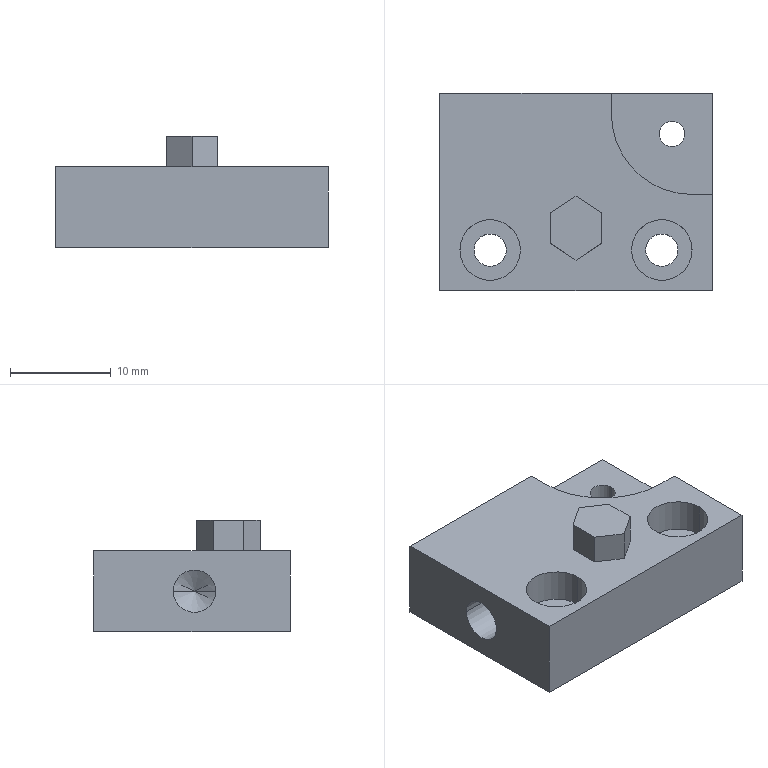Part | NX | 1 solid | 33 faces | box 27 x 19.5 x 11 mm | volume 3556 mm3 | plane 18 | cylinder 13 | cone 2 | commonest cylinder face diameters 3.2 x4 6 x4 2.5 x2 4.2 x2 16 x1
STEP:
#1=CARTESIAN_POINT('',(27.,0.,0.));
#2=VERTEX_POINT('',#1);
#3=CARTESIAN_POINT('',(0.,0.,0.));
#4=VERTEX_POINT('',#3);
#5=CARTESIAN_POINT('',(27.,0.,0.));
#6=DIRECTION('',(-1.,0.,0.));
#7=VECTOR('',#6,1000.);
#8=LINE('',#5,#7);
#9=EDGE_CURVE('',#2,#4,#8,.T.);
#10=ORIENTED_EDGE('',*,*,#9,.T.);
#11=CARTESIAN_POINT('',(0.,19.5,0.));
#12=VERTEX_POINT('',#11);
#13=CARTESIAN_POINT('',(0.,0.,0.));
#14=DIRECTION('',(0.,1.,0.));
#15=VECTOR('',#14,1000.);
#16=LINE('',#13,#15);
#17=EDGE_CURVE('',#4,#12,#16,.T.);
#18=ORIENTED_EDGE('',*,*,#17,.T.);
#19=CARTESIAN_POINT('',(27.,19.5,0.));
#20=VERTEX_POINT('',#19);
#21=CARTESIAN_POINT('',(0.,19.5,0.));
#22=DIRECTION('',(1.,0.,0.));
#23=VECTOR('',#22,1000.);
#24=LINE('',#21,#23);
#25=EDGE_CURVE('',#12,#20,#24,.T.);
#26=ORIENTED_EDGE('',*,*,#25,.T.);
#27=CARTESIAN_POINT('',(27.,19.5,0.));
#28=DIRECTION('',(0.,-1.,0.));
#29=VECTOR('',#28,1000.);
#30=LINE('',#27,#29);
#31=EDGE_CURVE('',#20,#2,#30,.T.);
#32=ORIENTED_EDGE('',*,*,#31,.T.);
#33=EDGE_LOOP('',(#10,#18,#26,#32));
#34=FACE_BOUND('',#33,.T.);
#35=CARTESIAN_POINT('',(6.6,4.,0.));
#36=VERTEX_POINT('',#35);
#37=CARTESIAN_POINT('',(3.4,4.,0.));
#38=VERTEX_POINT('',#37);
#39=CARTESIAN_POINT('',(5.,4.,0.));
#40=DIRECTION('',(0.,0.,-1.));
#41=DIRECTION('',(-1.,0.,0.));
#42=AXIS2_PLACEMENT_3D('',#39,#40,#41);
#43=CIRCLE('',#42,1.6);
#44=EDGE_CURVE('',#36,#38,#43,.T.);
#45=ORIENTED_EDGE('',*,*,#44,.F.);
#46=CARTESIAN_POINT('',(5.,4.,0.));
#47=DIRECTION('',(0.,0.,-1.));
#48=DIRECTION('',(-1.,0.,0.));
#49=AXIS2_PLACEMENT_3D('',#46,#47,#48);
#50=CIRCLE('',#49,1.6);
#51=EDGE_CURVE('',#38,#36,#50,.T.);
#52=ORIENTED_EDGE('',*,*,#51,.F.);
#53=EDGE_LOOP('',(#45,#52));
#54=FACE_BOUND('',#53,.T.);
#55=CARTESIAN_POINT('',(23.6,4.,0.));
#56=VERTEX_POINT('',#55);
#57=CARTESIAN_POINT('',(20.4,4.,0.));
#58=VERTEX_POINT('',#57);
#59=CARTESIAN_POINT('',(22.,4.,0.));
#60=DIRECTION('',(0.,0.,-1.));
#61=DIRECTION('',(-1.,0.,0.));
#62=AXIS2_PLACEMENT_3D('',#59,#60,#61);
#63=CIRCLE('',#62,1.6);
#64=EDGE_CURVE('',#56,#58,#63,.T.);
#65=ORIENTED_EDGE('',*,*,#64,.F.);
#66=CARTESIAN_POINT('',(22.,4.,0.));
#67=DIRECTION('',(0.,0.,-1.));
#68=DIRECTION('',(-1.,0.,0.));
#69=AXIS2_PLACEMENT_3D('',#66,#67,#68);
#70=CIRCLE('',#69,1.6);
#71=EDGE_CURVE('',#58,#56,#70,.T.);
#72=ORIENTED_EDGE('',*,*,#71,.F.);
#73=EDGE_LOOP('',(#65,#72));
#74=FACE_BOUND('',#73,.T.);
#75=CARTESIAN_POINT('',(24.25,15.5,0.));
#76=VERTEX_POINT('',#75);
#77=CARTESIAN_POINT('',(21.75,15.5,0.));
#78=VERTEX_POINT('',#77);
#79=CARTESIAN_POINT('',(23.,15.5,0.));
#80=DIRECTION('',(0.,0.,-1.));
#81=DIRECTION('',(-1.,0.,0.));
#82=AXIS2_PLACEMENT_3D('',#79,#80,#81);
#83=CIRCLE('',#82,1.25);
#84=EDGE_CURVE('',#76,#78,#83,.T.);
#85=ORIENTED_EDGE('',*,*,#84,.F.);
#86=CARTESIAN_POINT('',(23.,15.5,0.));
#87=DIRECTION('',(0.,0.,-1.));
#88=DIRECTION('',(-1.,0.,0.));
#89=AXIS2_PLACEMENT_3D('',#86,#87,#88);
#90=CIRCLE('',#89,1.25);
#91=EDGE_CURVE('',#78,#76,#90,.T.);
#92=ORIENTED_EDGE('',*,*,#91,.F.);
#93=EDGE_LOOP('',(#85,#92));
#94=FACE_BOUND('',#93,.T.);
#95=CARTESIAN_POINT('',(0.,0.,0.));
#96=DIRECTION('',(0.,0.,1.));
#97=DIRECTION('',(1.,0.,0.));
#98=AXIS2_PLACEMENT_3D('',#95,#96,#97);
#99=PLANE('',#98);
#100=ADVANCED_FACE('',(#34,#54,#74,#94),#99,.F.);
#101=ORIENTED_EDGE('',*,*,#9,.F.);
#102=CARTESIAN_POINT('',(27.,0.,8.));
#103=VERTEX_POINT('',#102);
#104=CARTESIAN_POINT('',(27.,0.,8.));
#105=DIRECTION('',(0.,0.,-1.));
#106=VECTOR('',#105,1000.);
#107=LINE('',#104,#106);
#108=EDGE_CURVE('',#103,#2,#107,.T.);
#109=ORIENTED_EDGE('',*,*,#108,.F.);
#110=CARTESIAN_POINT('',(0.,0.,8.));
#111=VERTEX_POINT('',#110);
#112=CARTESIAN_POINT('',(27.,0.,8.));
#113=DIRECTION('',(-1.,0.,0.));
#114=VECTOR('',#113,1000.);
#115=LINE('',#112,#114);
#116=EDGE_CURVE('',#103,#111,#115,.T.);
#117=ORIENTED_EDGE('',*,*,#116,.T.);
#118=CARTESIAN_POINT('',(0.,0.,8.));
#119=DIRECTION('',(0.,0.,-1.));
#120=VECTOR('',#119,1000.);
#121=LINE('',#118,#120);
#122=EDGE_CURVE('',#111,#4,#121,.T.);
#123=ORIENTED_EDGE('',*,*,#122,.T.);
#124=EDGE_LOOP('',(#101,#109,#117,#123));
#125=FACE_BOUND('',#124,.T.);
#126=CARTESIAN_POINT('',(0.,0.,0.));
#127=DIRECTION('',(0.,-1.,0.));
#128=DIRECTION('',(0.,0.,-1.));
#129=AXIS2_PLACEMENT_3D('',#126,#127,#128);
#130=PLANE('',#129);
#131=ADVANCED_FACE('',(#125),#130,.T.);
#132=ORIENTED_EDGE('',*,*,#17,.F.);
#133=ORIENTED_EDGE('',*,*,#122,.F.);
#134=CARTESIAN_POINT('',(0.,19.5,8.));
#135=VERTEX_POINT('',#134);
#136=CARTESIAN_POINT('',(0.,0.,8.));
#137=DIRECTION('',(0.,1.,0.));
#138=VECTOR('',#137,1000.);
#139=LINE('',#136,#138);
#140=EDGE_CURVE('',#111,#135,#139,.T.);
#141=ORIENTED_EDGE('',*,*,#140,.T.);
#142=CARTESIAN_POINT('',(0.,19.5,8.));
#143=DIRECTION('',(0.,0.,-1.));
#144=VECTOR('',#143,1000.);
#145=LINE('',#142,#144);
#146=EDGE_CURVE('',#135,#12,#145,.T.);
#147=ORIENTED_EDGE('',*,*,#146,.T.);
#148=EDGE_LOOP('',(#132,#133,#141,#147));
#149=FACE_BOUND('',#148,.T.);
#150=CARTESIAN_POINT('',(0.,11.6,4.));
#151=VERTEX_POINT('',#150);
#152=CARTESIAN_POINT('',(0.,7.4,4.));
#153=VERTEX_POINT('',#152);
#154=CARTESIAN_POINT('',(0.,9.5,4.));
#155=DIRECTION('',(-1.,0.,0.));
#156=DIRECTION('',(0.,-1.,0.));
#157=AXIS2_PLACEMENT_3D('',#154,#155,#156);
#158=CIRCLE('',#157,2.1);
#159=EDGE_CURVE('',#151,#153,#158,.T.);
#160=ORIENTED_EDGE('',*,*,#159,.F.);
#161=CARTESIAN_POINT('',(0.,9.5,4.));
#162=DIRECTION('',(-1.,0.,0.));
#163=DIRECTION('',(0.,-1.,0.));
#164=AXIS2_PLACEMENT_3D('',#161,#162,#163);
#165=CIRCLE('',#164,2.1);
#166=EDGE_CURVE('',#153,#151,#165,.T.);
#167=ORIENTED_EDGE('',*,*,#166,.F.);
#168=EDGE_LOOP('',(#160,#167));
#169=FACE_BOUND('',#168,.T.);
#170=CARTESIAN_POINT('',(0.,19.5,0.));
#171=DIRECTION('',(-1.,0.,0.));
#172=DIRECTION('',(0.,0.,1.));
#173=AXIS2_PLACEMENT_3D('',#170,#171,#172);
#174=PLANE('',#173);
#175=ADVANCED_FACE('',(#149,#169),#174,.T.);
#176=CARTESIAN_POINT('',(17.,19.5,5.));
#177=VERTEX_POINT('',#176);
#178=CARTESIAN_POINT('',(27.,19.5,5.));
#179=VERTEX_POINT('',#178);
#180=CARTESIAN_POINT('',(17.,19.5,5.));
#181=DIRECTION('',(1.,0.,0.));
#182=VECTOR('',#181,1000.);
#183=LINE('',#180,#182);
#184=EDGE_CURVE('',#177,#179,#183,.T.);
#185=ORIENTED_EDGE('',*,*,#184,.T.);
#186=CARTESIAN_POINT('',(27.,19.5,5.));
#187=DIRECTION('',(0.,0.,-1.));
#188=VECTOR('',#187,1000.);
#189=LINE('',#186,#188);
#190=EDGE_CURVE('',#179,#20,#189,.T.);
#191=ORIENTED_EDGE('',*,*,#190,.T.);
#192=ORIENTED_EDGE('',*,*,#25,.F.);
#193=ORIENTED_EDGE('',*,*,#146,.F.);
#194=CARTESIAN_POINT('',(17.,19.5,8.));
#195=VERTEX_POINT('',#194);
#196=CARTESIAN_POINT('',(0.,19.5,8.));
#197=DIRECTION('',(1.,0.,0.));
#198=VECTOR('',#197,1000.);
#199=LINE('',#196,#198);
#200=EDGE_CURVE('',#135,#195,#199,.T.);
#201=ORIENTED_EDGE('',*,*,#200,.T.);
#202=CARTESIAN_POINT('',(17.,19.5,5.));
#203=DIRECTION('',(0.,0.,1.));
#204=VECTOR('',#203,1000.);
#205=LINE('',#202,#204);
#206=EDGE_CURVE('',#177,#195,#205,.T.);
#207=ORIENTED_EDGE('',*,*,#206,.F.);
#208=EDGE_LOOP('',(#185,#191,#192,#193,#201,#207));
#209=FACE_BOUND('',#208,.T.);
#210=CARTESIAN_POINT('',(27.,19.5,0.));
#211=DIRECTION('',(0.,1.,0.));
#212=DIRECTION('',(1.,0.,0.));
#213=AXIS2_PLACEMENT_3D('',#210,#211,#212);
#214=PLANE('',#213);
#215=ADVANCED_FACE('',(#209),#214,.T.);
#216=CARTESIAN_POINT('',(27.,9.5,5.));
#217=VERTEX_POINT('',#216);
#218=CARTESIAN_POINT('',(27.,9.5,5.));
#219=DIRECTION('',(0.,1.,0.));
#220=VECTOR('',#219,1000.);
#221=LINE('',#218,#220);
#222=EDGE_CURVE('',#217,#179,#221,.T.);
#223=ORIENTED_EDGE('',*,*,#222,.T.);
#224=ORIENTED_EDGE('',*,*,#184,.F.);
#225=CARTESIAN_POINT('',(17.,17.5,5.));
#226=VERTEX_POINT('',#225);
#227=CARTESIAN_POINT('',(17.,17.5,5.));
#228=DIRECTION('',(0.,1.,0.));
#229=VECTOR('',#228,1000.);
#230=LINE('',#227,#229);
#231=EDGE_CURVE('',#226,#177,#230,.T.);
#232=ORIENTED_EDGE('',*,*,#231,.F.);
#233=CARTESIAN_POINT('',(25.,9.5,5.));
#234=VERTEX_POINT('',#233);
#235=CARTESIAN_POINT('',(25.,17.5,5.));
#236=DIRECTION('',(0.,0.,-1.));
#237=DIRECTION('',(0.,-1.,0.));
#238=AXIS2_PLACEMENT_3D('',#235,#236,#237);
#239=CIRCLE('',#238,8.);
#240=EDGE_CURVE('',#234,#226,#239,.T.);
#241=ORIENTED_EDGE('',*,*,#240,.F.);
#242=CARTESIAN_POINT('',(27.,9.5,5.));
#243=DIRECTION('',(-1.,0.,0.));
#244=VECTOR('',#243,1000.);
#245=LINE('',#242,#244);
#246=EDGE_CURVE('',#217,#234,#245,.T.);
#247=ORIENTED_EDGE('',*,*,#246,.F.);
#248=EDGE_LOOP('',(#223,#224,#232,#241,#247));
#249=FACE_BOUND('',#248,.T.);
#250=CARTESIAN_POINT('',(24.25,15.5,5.));
#251=VERTEX_POINT('',#250);
#252=CARTESIAN_POINT('',(21.75,15.5,5.));
#253=VERTEX_POINT('',#252);
#254=CARTESIAN_POINT('',(23.,15.5,5.));
#255=DIRECTION('',(0.,0.,1.));
#256=DIRECTION('',(1.,0.,0.));
#257=AXIS2_PLACEMENT_3D('',#254,#255,#256);
#258=CIRCLE('',#257,1.25);
#259=EDGE_CURVE('',#251,#253,#258,.T.);
#260=ORIENTED_EDGE('',*,*,#259,.F.);
#261=CARTESIAN_POINT('',(23.,15.5,5.));
#262=DIRECTION('',(0.,0.,1.));
#263=DIRECTION('',(1.,0.,0.));
#264=AXIS2_PLACEMENT_3D('',#261,#262,#263);
#265=CIRCLE('',#264,1.25);
#266=EDGE_CURVE('',#253,#251,#265,.T.);
#267=ORIENTED_EDGE('',*,*,#266,.F.);
#268=EDGE_LOOP('',(#260,#267));
#269=FACE_BOUND('',#268,.T.);
#270=CARTESIAN_POINT('',(0.,0.,5.));
#271=DIRECTION('',(0.,0.,1.));
#272=DIRECTION('',(1.,0.,0.));
#273=AXIS2_PLACEMENT_3D('',#270,#271,#272);
#274=PLANE('',#273);
#275=ADVANCED_FACE('',(#249,#269),#274,.T.);
#276=ORIENTED_EDGE('',*,*,#222,.F.);
#277=CARTESIAN_POINT('',(27.,9.5,8.));
#278=VERTEX_POINT('',#277);
#279=CARTESIAN_POINT('',(27.,9.5,5.));
#280=DIRECTION('',(0.,0.,1.));
#281=VECTOR('',#280,1000.);
#282=LINE('',#279,#281);
#283=EDGE_CURVE('',#217,#278,#282,.T.);
#284=ORIENTED_EDGE('',*,*,#283,.T.);
#285=CARTESIAN_POINT('',(27.,9.5,8.));
#286=DIRECTION('',(0.,-1.,0.));
#287=VECTOR('',#286,1000.);
#288=LINE('',#285,#287);
#289=EDGE_CURVE('',#278,#103,#288,.T.);
#290=ORIENTED_EDGE('',*,*,#289,.T.);
#291=ORIENTED_EDGE('',*,*,#108,.T.);
#292=ORIENTED_EDGE('',*,*,#31,.F.);
#293=ORIENTED_EDGE('',*,*,#190,.F.);
#294=EDGE_LOOP('',(#276,#284,#290,#291,#292,#293));
#295=FACE_BOUND('',#294,.T.);
#296=CARTESIAN_POINT('',(27.,0.,0.));
#297=DIRECTION('',(1.,0.,0.));
#298=DIRECTION('',(0.,1.,0.));
#299=AXIS2_PLACEMENT_3D('',#296,#297,#298);
#300=PLANE('',#299);
#301=ADVANCED_FACE('',(#295),#300,.T.);
#302=CARTESIAN_POINT('',(17.,17.5,8.));
#303=VERTEX_POINT('',#302);
#304=CARTESIAN_POINT('',(17.,17.5,8.));
#305=DIRECTION('',(0.,1.,0.));
#306=VECTOR('',#305,1000.);
#307=LINE('',#304,#306);
#308=EDGE_CURVE('',#303,#195,#307,.T.);
#309=ORIENTED_EDGE('',*,*,#308,.T.);
#310=ORIENTED_EDGE('',*,*,#200,.F.);
#311=ORIENTED_EDGE('',*,*,#140,.F.);
#312=ORIENTED_EDGE('',*,*,#116,.F.);
#313=ORIENTED_EDGE('',*,*,#289,.F.);
#314=CARTESIAN_POINT('',(25.,9.5,8.));
#315=VERTEX_POINT('',#314);
#316=CARTESIAN_POINT('',(25.,9.5,8.));
#317=DIRECTION('',(1.,0.,0.));
#318=VECTOR('',#317,1000.);
#319=LINE('',#316,#318);
#320=EDGE_CURVE('',#315,#278,#319,.T.);
#321=ORIENTED_EDGE('',*,*,#320,.F.);
#322=CARTESIAN_POINT('',(25.,17.5,8.));
#323=DIRECTION('',(0.,0.,1.));
#324=DIRECTION('',(-1.,0.,0.));
#325=AXIS2_PLACEMENT_3D('',#322,#323,#324);
#326=CIRCLE('',#325,8.);
#327=EDGE_CURVE('',#303,#315,#326,.T.);
#328=ORIENTED_EDGE('',*,*,#327,.F.);
#329=EDGE_LOOP('',(#309,#310,#311,#312,#313,#321,#328));
#330=FACE_BOUND('',#329,.T.);
#331=CARTESIAN_POINT('',(8.,4.,8.));
#332=VERTEX_POINT('',#331);
#333=CARTESIAN_POINT('',(2.,4.,8.));
#334=VERTEX_POINT('',#333);
#335=CARTESIAN_POINT('',(5.,4.,8.));
#336=DIRECTION('',(0.,0.,1.));
#337=DIRECTION('',(1.,0.,0.));
#338=AXIS2_PLACEMENT_3D('',#335,#336,#337);
#339=CIRCLE('',#338,3.);
#340=EDGE_CURVE('',#332,#334,#339,.T.);
#341=ORIENTED_EDGE('',*,*,#340,.F.);
#342=CARTESIAN_POINT('',(5.,4.,8.));
#343=DIRECTION('',(0.,0.,1.));
#344=DIRECTION('',(1.,0.,0.));
#345=AXIS2_PLACEMENT_3D('',#342,#343,#344);
#346=CIRCLE('',#345,3.);
#347=EDGE_CURVE('',#334,#332,#346,.T.);
#348=ORIENTED_EDGE('',*,*,#347,.F.);
#349=EDGE_LOOP('',(#341,#348));
#350=FACE_BOUND('',#349,.T.);
#351=CARTESIAN_POINT('',(19.,4.,8.));
#352=VERTEX_POINT('',#351);
#353=CARTESIAN_POINT('',(25.,4.,8.));
#354=VERTEX_POINT('',#353);
#355=CARTESIAN_POINT('',(22.,4.,8.));
#356=DIRECTION('',(0.,0.,1.));
#357=DIRECTION('',(1.,0.,0.));
#358=AXIS2_PLACEMENT_3D('',#355,#356,#357);
#359=CIRCLE('',#358,3.);
#360=EDGE_CURVE('',#352,#354,#359,.T.);
#361=ORIENTED_EDGE('',*,*,#360,.F.);
#362=CARTESIAN_POINT('',(22.,4.,8.));
#363=DIRECTION('',(0.,0.,1.));
#364=DIRECTION('',(1.,0.,0.));
#365=AXIS2_PLACEMENT_3D('',#362,#363,#364);
#366=CIRCLE('',#365,3.);
#367=EDGE_CURVE('',#354,#352,#366,.T.);
#368=ORIENTED_EDGE('',*,*,#367,.F.);
#369=EDGE_LOOP('',(#361,#368));
#370=FACE_BOUND('',#369,.T.);
#371=CARTESIAN_POINT('',(13.5,9.317,8.));
#372=VERTEX_POINT('',#371);
#373=CARTESIAN_POINT('',(11.,7.658,8.));
#374=VERTEX_POINT('',#373);
#375=CARTESIAN_POINT('',(13.5,9.317,8.));
#376=DIRECTION('',(-0.8333,-0.5528,0.));
#377=VECTOR('',#376,1000.);
#378=LINE('',#375,#377);
#379=EDGE_CURVE('',#372,#374,#378,.T.);
#380=ORIENTED_EDGE('',*,*,#379,.F.);
#381=CARTESIAN_POINT('',(16.,7.658,8.));
#382=VERTEX_POINT('',#381);
#383=CARTESIAN_POINT('',(16.,7.658,8.));
#384=DIRECTION('',(-0.8333,0.5528,0.));
#385=VECTOR('',#384,1000.);
#386=LINE('',#383,#385);
#387=EDGE_CURVE('',#382,#372,#386,.T.);
#388=ORIENTED_EDGE('',*,*,#387,.F.);
#389=CARTESIAN_POINT('',(16.,4.658,8.));
#390=VERTEX_POINT('',#389);
#391=CARTESIAN_POINT('',(16.,7.658,8.));
#392=DIRECTION('',(0.,-1.,0.));
#393=VECTOR('',#392,1000.);
#394=LINE('',#391,#393);
#395=EDGE_CURVE('',#382,#390,#394,.T.);
#396=ORIENTED_EDGE('',*,*,#395,.T.);
#397=CARTESIAN_POINT('',(13.5,3.,8.));
#398=VERTEX_POINT('',#397);
#399=CARTESIAN_POINT('',(13.5,3.,8.));
#400=DIRECTION('',(0.8333,0.5528,0.));
#401=VECTOR('',#400,1000.);
#402=LINE('',#399,#401);
#403=EDGE_CURVE('',#398,#390,#402,.T.);
#404=ORIENTED_EDGE('',*,*,#403,.F.);
#405=CARTESIAN_POINT('',(11.,4.658,8.));
#406=VERTEX_POINT('',#405);
#407=CARTESIAN_POINT('',(11.,4.658,8.));
#408=DIRECTION('',(0.8333,-0.5528,0.));
#409=VECTOR('',#408,1000.);
#410=LINE('',#407,#409);
#411=EDGE_CURVE('',#406,#398,#410,.T.);
#412=ORIENTED_EDGE('',*,*,#411,.F.);
#413=CARTESIAN_POINT('',(11.,4.658,8.));
#414=DIRECTION('',(0.,1.,0.));
#415=VECTOR('',#414,1000.);
#416=LINE('',#413,#415);
#417=EDGE_CURVE('',#406,#374,#416,.T.);
#418=ORIENTED_EDGE('',*,*,#417,.T.);
#419=EDGE_LOOP('',(#380,#388,#396,#404,#412,#418));
#420=FACE_BOUND('',#419,.T.);
#421=CARTESIAN_POINT('',(0.,0.,8.));
#422=DIRECTION('',(0.,0.,1.));
#423=DIRECTION('',(1.,0.,0.));
#424=AXIS2_PLACEMENT_3D('',#421,#422,#423);
#425=PLANE('',#424);
#426=ADVANCED_FACE('',(#330,#350,#370,#420),#425,.T.);
#427=ORIENTED_EDGE('',*,*,#308,.F.);
#428=CARTESIAN_POINT('',(17.,17.5,8.));
#429=DIRECTION('',(0.,0.,1.));
#430=VECTOR('',#429,1000.);
#431=LINE('',#428,#430);
#432=EDGE_CURVE('',#226,#303,#431,.T.);
#433=ORIENTED_EDGE('',*,*,#432,.F.);
#434=ORIENTED_EDGE('',*,*,#231,.T.);
#435=ORIENTED_EDGE('',*,*,#206,.T.);
#436=EDGE_LOOP('',(#427,#433,#434,#435));
#437=FACE_BOUND('',#436,.T.);
#438=CARTESIAN_POINT('',(17.,19.5,8.));
#439=DIRECTION('',(-1.,0.,0.));
#440=DIRECTION('',(0.,0.,1.));
#441=AXIS2_PLACEMENT_3D('',#438,#439,#440);
#442=PLANE('',#441);
#443=ADVANCED_FACE('',(#437),#442,.F.);
#444=ORIENTED_EDGE('',*,*,#327,.T.);
#445=CARTESIAN_POINT('',(25.,9.5,5.));
#446=DIRECTION('',(0.,0.,1.));
#447=VECTOR('',#446,1000.);
#448=LINE('',#445,#447);
#449=EDGE_CURVE('',#234,#315,#448,.T.);
#450=ORIENTED_EDGE('',*,*,#449,.F.);
#451=ORIENTED_EDGE('',*,*,#240,.T.);
#452=ORIENTED_EDGE('',*,*,#432,.T.);
#453=EDGE_LOOP('',(#444,#450,#451,#452));
#454=FACE_BOUND('',#453,.T.);
#455=CARTESIAN_POINT('',(25.,17.5,8.));
#456=DIRECTION('',(0.,0.,1.));
#457=DIRECTION('',(1.,0.,0.));
#458=AXIS2_PLACEMENT_3D('',#455,#456,#457);
#459=CYLINDRICAL_SURFACE('',#458,8.);
#460=ADVANCED_FACE('',(#454),#459,.F.);
#461=ORIENTED_EDGE('',*,*,#320,.T.);
#462=ORIENTED_EDGE('',*,*,#283,.F.);
#463=ORIENTED_EDGE('',*,*,#246,.T.);
#464=ORIENTED_EDGE('',*,*,#449,.T.);
#465=EDGE_LOOP('',(#461,#462,#463,#464));
#466=FACE_BOUND('',#465,.T.);
#467=CARTESIAN_POINT('',(25.,9.5,8.));
#468=DIRECTION('',(0.,-1.,0.));
#469=DIRECTION('',(0.,0.,-1.));
#470=AXIS2_PLACEMENT_3D('',#467,#468,#469);
#471=PLANE('',#470);
#472=ADVANCED_FACE('',(#466),#471,.F.);
#473=CARTESIAN_POINT('',(2.,4.,4.7));
#474=VERTEX_POINT('',#473);
#475=CARTESIAN_POINT('',(8.,4.,4.7));
#476=VERTEX_POINT('',#475);
#477=CARTESIAN_POINT('',(5.,4.,4.7));
#478=DIRECTION('',(0.,0.,-1.));
#479=DIRECTION('',(-1.,0.,0.));
#480=AXIS2_PLACEMENT_3D('',#477,#478,#479);
#481=CIRCLE('',#480,3.);
#482=EDGE_CURVE('',#474,#476,#481,.T.);
#483=ORIENTED_EDGE('',*,*,#482,.T.);
#484=CARTESIAN_POINT('',(8.,4.,-1.24));
#485=DIRECTION('',(0.,0.,1.));
#486=VECTOR('',#485,1000.);
#487=LINE('',#484,#486);
#488=EDGE_CURVE('',#332,#476,#487,.F.);
#489=ORIENTED_EDGE('',*,*,#488,.F.);
#490=ORIENTED_EDGE('',*,*,#340,.T.);
#491=CARTESIAN_POINT('',(2.,4.,-1.24));
#492=DIRECTION('',(0.,0.,1.));
#493=VECTOR('',#492,1000.);
#494=LINE('',#491,#493);
#495=EDGE_CURVE('',#334,#474,#494,.F.);
#496=ORIENTED_EDGE('',*,*,#495,.T.);
#497=EDGE_LOOP('',(#483,#489,#490,#496));
#498=FACE_BOUND('',#497,.T.);
#499=CARTESIAN_POINT('',(5.,4.,-1.24));
#500=DIRECTION('',(0.,0.,1.));
#501=DIRECTION('',(-1.,0.,0.));
#502=AXIS2_PLACEMENT_3D('',#499,#500,#501);
#503=CYLINDRICAL_SURFACE('',#502,3.);
#504=ADVANCED_FACE('',(#498),#503,.F.);
#505=ORIENTED_EDGE('',*,*,#84,.T.);
#506=CARTESIAN_POINT('',(21.75,15.5,-2.455));
#507=DIRECTION('',(0.,0.,1.));
#508=VECTOR('',#507,1000.);
#509=LINE('',#506,#508);
#510=EDGE_CURVE('',#253,#78,#509,.F.);
#511=ORIENTED_EDGE('',*,*,#510,.F.);
#512=ORIENTED_EDGE('',*,*,#266,.T.);
#513=CARTESIAN_POINT('',(24.25,15.5,-2.455));
#514=DIRECTION('',(0.,0.,1.));
#515=VECTOR('',#514,1000.);
#516=LINE('',#513,#515);
#517=EDGE_CURVE('',#251,#76,#516,.F.);
#518=ORIENTED_EDGE('',*,*,#517,.T.);
#519=EDGE_LOOP('',(#505,#511,#512,#518));
#520=FACE_BOUND('',#519,.T.);
#521=CARTESIAN_POINT('',(23.,15.5,-2.455));
#522=DIRECTION('',(0.,0.,1.));
#523=DIRECTION('',(-1.,0.,0.));
#524=AXIS2_PLACEMENT_3D('',#521,#522,#523);
#525=CYLINDRICAL_SURFACE('',#524,1.25);
#526=ADVANCED_FACE('',(#520),#525,.F.);
#527=ORIENTED_EDGE('',*,*,#482,.F.);
#528=CARTESIAN_POINT('',(5.,4.,4.7));
#529=DIRECTION('',(0.,0.,-1.));
#530=DIRECTION('',(-1.,0.,0.));
#531=AXIS2_PLACEMENT_3D('',#528,#529,#530);
#532=CIRCLE('',#531,3.);
#533=EDGE_CURVE('',#476,#474,#532,.T.);
#534=ORIENTED_EDGE('',*,*,#533,.F.);
#535=EDGE_LOOP('',(#527,#534));
#536=FACE_BOUND('',#535,.T.);
#537=CARTESIAN_POINT('',(6.6,4.,4.7));
#538=VERTEX_POINT('',#537);
#539=CARTESIAN_POINT('',(3.4,4.,4.7));
#540=VERTEX_POINT('',#539);
#541=CARTESIAN_POINT('',(5.,4.,4.7));
#542=DIRECTION('',(0.,0.,1.));
#543=DIRECTION('',(-1.,0.,0.));
#544=AXIS2_PLACEMENT_3D('',#541,#542,#543);
#545=CIRCLE('',#544,1.6);
#546=EDGE_CURVE('',#538,#540,#545,.T.);
#547=ORIENTED_EDGE('',*,*,#546,.F.);
#548=CARTESIAN_POINT('',(5.,4.,4.7));
#549=DIRECTION('',(0.,0.,1.));
#550=DIRECTION('',(-1.,0.,0.));
#551=AXIS2_PLACEMENT_3D('',#548,#549,#550);
#552=CIRCLE('',#551,1.6);
#553=EDGE_CURVE('',#540,#538,#552,.T.);
#554=ORIENTED_EDGE('',*,*,#553,.F.);
#555=EDGE_LOOP('',(#547,#554));
#556=FACE_BOUND('',#555,.T.);
#557=CARTESIAN_POINT('',(5.,4.,4.7));
#558=DIRECTION('',(0.,0.,1.));
#559=DIRECTION('',(1.,0.,0.));
#560=AXIS2_PLACEMENT_3D('',#557,#558,#559);
#561=PLANE('',#560);
#562=ADVANCED_FACE('',(#536,#556),#561,.T.);
#563=ORIENTED_EDGE('',*,*,#546,.T.);
#564=CARTESIAN_POINT('',(3.4,4.,-1.24));
#565=DIRECTION('',(0.,0.,1.));
#566=VECTOR('',#565,1000.);
#567=LINE('',#564,#566);
#568=EDGE_CURVE('',#540,#38,#567,.F.);
#569=ORIENTED_EDGE('',*,*,#568,.T.);
#570=ORIENTED_EDGE('',*,*,#51,.T.);
#571=CARTESIAN_POINT('',(6.6,4.,-1.24));
#572=DIRECTION('',(0.,0.,1.));
#573=VECTOR('',#572,1000.);
#574=LINE('',#571,#573);
#575=EDGE_CURVE('',#538,#36,#574,.F.);
#576=ORIENTED_EDGE('',*,*,#575,.F.);
#577=EDGE_LOOP('',(#563,#569,#570,#576));
#578=FACE_BOUND('',#577,.T.);
#579=CARTESIAN_POINT('',(5.,4.,-1.24));
#580=DIRECTION('',(0.,0.,1.));
#581=DIRECTION('',(-1.,0.,0.));
#582=AXIS2_PLACEMENT_3D('',#579,#580,#581);
#583=CYLINDRICAL_SURFACE('',#582,1.6);
#584=ADVANCED_FACE('',(#578),#583,.F.);
#585=CARTESIAN_POINT('',(11.,7.658,11.));
#586=VERTEX_POINT('',#585);
#587=CARTESIAN_POINT('',(13.5,9.317,11.));
#588=VERTEX_POINT('',#587);
#589=CARTESIAN_POINT('',(11.,7.658,11.));
#590=DIRECTION('',(0.8333,0.5528,0.));
#591=VECTOR('',#590,1000.);
#592=LINE('',#589,#591);
#593=EDGE_CURVE('',#586,#588,#592,.T.);
#594=ORIENTED_EDGE('',*,*,#593,.F.);
#595=CARTESIAN_POINT('',(11.,4.658,11.));
#596=VERTEX_POINT('',#595);
#597=CARTESIAN_POINT('',(11.,4.658,11.));
#598=DIRECTION('',(0.,1.,0.));
#599=VECTOR('',#598,1000.);
#600=LINE('',#597,#599);
#601=EDGE_CURVE('',#596,#586,#600,.T.);
#602=ORIENTED_EDGE('',*,*,#601,.F.);
#603=CARTESIAN_POINT('',(13.5,3.,11.));
#604=VERTEX_POINT('',#603);
#605=CARTESIAN_POINT('',(13.5,3.,11.));
#606=DIRECTION('',(-0.8333,0.5528,0.));
#607=VECTOR('',#606,1000.);
#608=LINE('',#605,#607);
#609=EDGE_CURVE('',#604,#596,#608,.T.);
#610=ORIENTED_EDGE('',*,*,#609,.F.);
#611=CARTESIAN_POINT('',(16.,4.658,11.));
#612=VERTEX_POINT('',#611);
#613=CARTESIAN_POINT('',(16.,4.658,11.));
#614=DIRECTION('',(-0.8333,-0.5528,0.));
#615=VECTOR('',#614,1000.);
#616=LINE('',#613,#615);
#617=EDGE_CURVE('',#612,#604,#616,.T.);
#618=ORIENTED_EDGE('',*,*,#617,.F.);
#619=CARTESIAN_POINT('',(16.,7.658,11.));
#620=VERTEX_POINT('',#619);
#621=CARTESIAN_POINT('',(16.,7.658,11.));
#622=DIRECTION('',(0.,-1.,0.));
#623=VECTOR('',#622,1000.);
#624=LINE('',#621,#623);
#625=EDGE_CURVE('',#620,#612,#624,.T.);
#626=ORIENTED_EDGE('',*,*,#625,.F.);
#627=CARTESIAN_POINT('',(13.5,9.317,11.));
#628=DIRECTION('',(0.8333,-0.5528,0.));
#629=VECTOR('',#628,1000.);
#630=LINE('',#627,#629);
#631=EDGE_CURVE('',#588,#620,#630,.T.);
#632=ORIENTED_EDGE('',*,*,#631,.F.);
#633=EDGE_LOOP('',(#594,#602,#610,#618,#626,#632));
#634=FACE_BOUND('',#633,.T.);
#635=CARTESIAN_POINT('',(0.,0.,11.));
#636=DIRECTION('',(0.,0.,1.));
#637=DIRECTION('',(1.,0.,0.));
#638=AXIS2_PLACEMENT_3D('',#635,#636,#637);
#639=PLANE('',#638);
#640=ADVANCED_FACE('',(#634),#639,.T.);
#641=ORIENTED_EDGE('',*,*,#360,.T.);
#642=CARTESIAN_POINT('',(25.,4.,4.7));
#643=VERTEX_POINT('',#642);
#644=CARTESIAN_POINT('',(25.,4.,-1.24));
#645=DIRECTION('',(0.,0.,1.));
#646=VECTOR('',#645,1000.);
#647=LINE('',#644,#646);
#648=EDGE_CURVE('',#354,#643,#647,.F.);
#649=ORIENTED_EDGE('',*,*,#648,.T.);
#650=CARTESIAN_POINT('',(19.,4.,4.7));
#651=VERTEX_POINT('',#650);
#652=CARTESIAN_POINT('',(22.,4.,4.7));
#653=DIRECTION('',(0.,0.,-1.));
#654=DIRECTION('',(1.,0.,0.));
#655=AXIS2_PLACEMENT_3D('',#652,#653,#654);
#656=CIRCLE('',#655,3.);
#657=EDGE_CURVE('',#643,#651,#656,.T.);
#658=ORIENTED_EDGE('',*,*,#657,.T.);
#659=CARTESIAN_POINT('',(19.,4.,-1.24));
#660=DIRECTION('',(0.,0.,1.));
#661=VECTOR('',#660,1000.);
#662=LINE('',#659,#661);
#663=EDGE_CURVE('',#352,#651,#662,.F.);
#664=ORIENTED_EDGE('',*,*,#663,.F.);
#665=EDGE_LOOP('',(#641,#649,#658,#664));
#666=FACE_BOUND('',#665,.T.);
#667=CARTESIAN_POINT('',(22.,4.,-1.24));
#668=DIRECTION('',(0.,0.,1.));
#669=DIRECTION('',(-1.,0.,0.));
#670=AXIS2_PLACEMENT_3D('',#667,#668,#669);
#671=CYLINDRICAL_SURFACE('',#670,3.);
#672=ADVANCED_FACE('',(#666),#671,.F.);
#673=ORIENTED_EDGE('',*,*,#159,.T.);
#674=CARTESIAN_POINT('',(12.6,7.4,4.));
#675=VERTEX_POINT('',#674);
#676=CARTESIAN_POINT('',(14.555,7.4,4.));
#677=DIRECTION('',(-1.,0.,0.));
#678=VECTOR('',#677,1000.);
#679=LINE('',#676,#678);
#680=EDGE_CURVE('',#675,#153,#679,.T.);
#681=ORIENTED_EDGE('',*,*,#680,.F.);
#682=CARTESIAN_POINT('',(12.6,11.6,4.));
#683=VERTEX_POINT('',#682);
#684=CARTESIAN_POINT('',(12.6,9.5,4.));
#685=DIRECTION('',(1.,0.,0.));
#686=DIRECTION('',(0.,-1.,0.));
#687=AXIS2_PLACEMENT_3D('',#684,#685,#686);
#688=CIRCLE('',#687,2.1);
#689=EDGE_CURVE('',#675,#683,#688,.T.);
#690=ORIENTED_EDGE('',*,*,#689,.T.);
#691=CARTESIAN_POINT('',(14.555,11.6,4.));
#692=DIRECTION('',(-1.,0.,0.));
#693=VECTOR('',#692,1000.);
#694=LINE('',#691,#693);
#695=EDGE_CURVE('',#683,#151,#694,.T.);
#696=ORIENTED_EDGE('',*,*,#695,.T.);
#697=EDGE_LOOP('',(#673,#681,#690,#696));
#698=FACE_BOUND('',#697,.T.);
#699=CARTESIAN_POINT('',(14.555,9.5,4.));
#700=DIRECTION('',(-1.,0.,0.));
#701=DIRECTION('',(0.,1.,0.));
#702=AXIS2_PLACEMENT_3D('',#699,#700,#701);
#703=CYLINDRICAL_SURFACE('',#702,2.1);
#704=ADVANCED_FACE('',(#698),#703,.F.);
#705=ORIENTED_EDGE('',*,*,#657,.F.);
#706=CARTESIAN_POINT('',(22.,4.,4.7));
#707=DIRECTION('',(0.,0.,-1.));
#708=DIRECTION('',(1.,0.,0.));
#709=AXIS2_PLACEMENT_3D('',#706,#707,#708);
#710=CIRCLE('',#709,3.);
#711=EDGE_CURVE('',#651,#643,#710,.T.);
#712=ORIENTED_EDGE('',*,*,#711,.F.);
#713=EDGE_LOOP('',(#705,#712));
#714=FACE_BOUND('',#713,.T.);
#715=CARTESIAN_POINT('',(23.6,4.,4.7));
#716=VERTEX_POINT('',#715);
#717=CARTESIAN_POINT('',(20.4,4.,4.7));
#718=VERTEX_POINT('',#717);
#719=CARTESIAN_POINT('',(22.,4.,4.7));
#720=DIRECTION('',(0.,0.,1.));
#721=DIRECTION('',(-1.,0.,0.));
#722=AXIS2_PLACEMENT_3D('',#719,#720,#721);
#723=CIRCLE('',#722,1.6);
#724=EDGE_CURVE('',#716,#718,#723,.T.);
#725=ORIENTED_EDGE('',*,*,#724,.F.);
#726=CARTESIAN_POINT('',(22.,4.,4.7));
#727=DIRECTION('',(0.,0.,1.));
#728=DIRECTION('',(-1.,0.,0.));
#729=AXIS2_PLACEMENT_3D('',#726,#727,#728);
#730=CIRCLE('',#729,1.6);
#731=EDGE_CURVE('',#718,#716,#730,.T.);
#732=ORIENTED_EDGE('',*,*,#731,.F.);
#733=EDGE_LOOP('',(#725,#732));
#734=FACE_BOUND('',#733,.T.);
#735=CARTESIAN_POINT('',(22.,4.,4.7));
#736=DIRECTION('',(0.,0.,1.));
#737=DIRECTION('',(1.,0.,0.));
#738=AXIS2_PLACEMENT_3D('',#735,#736,#737);
#739=PLANE('',#738);
#740=ADVANCED_FACE('',(#714,#734),#739,.T.);
#741=ORIENTED_EDGE('',*,*,#64,.T.);
#742=CARTESIAN_POINT('',(20.4,4.,-1.24));
#743=DIRECTION('',(0.,0.,1.));
#744=VECTOR('',#743,1000.);
#745=LINE('',#742,#744);
#746=EDGE_CURVE('',#718,#58,#745,.F.);
#747=ORIENTED_EDGE('',*,*,#746,.F.);
#748=ORIENTED_EDGE('',*,*,#731,.T.);
#749=CARTESIAN_POINT('',(23.6,4.,-1.24));
#750=DIRECTION('',(0.,0.,1.));
#751=VECTOR('',#750,1000.);
#752=LINE('',#749,#751);
#753=EDGE_CURVE('',#716,#56,#752,.F.);
#754=ORIENTED_EDGE('',*,*,#753,.T.);
#755=EDGE_LOOP('',(#741,#747,#748,#754));
#756=FACE_BOUND('',#755,.T.);
#757=CARTESIAN_POINT('',(22.,4.,-1.24));
#758=DIRECTION('',(0.,0.,1.));
#759=DIRECTION('',(-1.,0.,0.));
#760=AXIS2_PLACEMENT_3D('',#757,#758,#759);
#761=CYLINDRICAL_SURFACE('',#760,1.6);
#762=ADVANCED_FACE('',(#756),#761,.F.);
#763=CARTESIAN_POINT('',(13.862,9.5,4.));
#764=VERTEX_POINT('',#763);
#765=CARTESIAN_POINT('',(13.218,8.429,4.));
#766=DIRECTION('',(-0.515,-0.8572,0.));
#767=VECTOR('',#766,1000.);
#768=LINE('',#765,#767);
#769=EDGE_CURVE('',#675,#764,#768,.F.);
#770=ORIENTED_EDGE('',*,*,#769,.F.);
#771=CARTESIAN_POINT('',(12.6,9.5,4.));
#772=DIRECTION('',(1.,0.,0.));
#773=DIRECTION('',(0.,-1.,0.));
#774=AXIS2_PLACEMENT_3D('',#771,#772,#773);
#775=CIRCLE('',#774,2.1);
#776=EDGE_CURVE('',#683,#675,#775,.T.);
#777=ORIENTED_EDGE('',*,*,#776,.F.);
#778=CARTESIAN_POINT('',(13.218,10.571,4.));
#779=DIRECTION('',(-0.515,0.8572,0.));
#780=VECTOR('',#779,1000.);
#781=LINE('',#778,#780);
#782=EDGE_CURVE('',#683,#764,#781,.F.);
#783=ORIENTED_EDGE('',*,*,#782,.T.);
#784=EDGE_LOOP('',(#770,#777,#783));
#785=FACE_BOUND('',#784,.T.);
#786=CARTESIAN_POINT('',(13.218,9.5,4.));
#787=DIRECTION('',(-1.,0.,0.));
#788=DIRECTION('',(0.,1.,0.));
#789=AXIS2_PLACEMENT_3D('',#786,#787,#788);
#790=CONICAL_SURFACE('',#789,1.071,1.03);
#791=ADVANCED_FACE('',(#785),#790,.F.);
#792=ORIENTED_EDGE('',*,*,#379,.T.);
#793=CARTESIAN_POINT('',(11.,7.658,11.));
#794=DIRECTION('',(0.,0.,-1.));
#795=VECTOR('',#794,1000.);
#796=LINE('',#793,#795);
#797=EDGE_CURVE('',#586,#374,#796,.T.);
#798=ORIENTED_EDGE('',*,*,#797,.F.);
#799=ORIENTED_EDGE('',*,*,#593,.T.);
#800=CARTESIAN_POINT('',(13.5,9.317,11.));
#801=DIRECTION('',(0.,0.,-1.));
#802=VECTOR('',#801,1000.);
#803=LINE('',#800,#802);
#804=EDGE_CURVE('',#588,#372,#803,.T.);
#805=ORIENTED_EDGE('',*,*,#804,.T.);
#806=EDGE_LOOP('',(#792,#798,#799,#805));
#807=FACE_BOUND('',#806,.T.);
#808=CARTESIAN_POINT('',(13.5,9.317,8.));
#809=DIRECTION('',(-0.5528,0.8333,0.));
#810=DIRECTION('',(0.,0.,1.));
#811=AXIS2_PLACEMENT_3D('',#808,#809,#810);
#812=PLANE('',#811);
#813=ADVANCED_FACE('',(#807),#812,.T.);
#814=ORIENTED_EDGE('',*,*,#387,.T.);
#815=ORIENTED_EDGE('',*,*,#804,.F.);
#816=ORIENTED_EDGE('',*,*,#631,.T.);
#817=CARTESIAN_POINT('',(16.,7.658,11.));
#818=DIRECTION('',(0.,0.,-1.));
#819=VECTOR('',#818,1000.);
#820=LINE('',#817,#819);
#821=EDGE_CURVE('',#620,#382,#820,.T.);
#822=ORIENTED_EDGE('',*,*,#821,.T.);
#823=EDGE_LOOP('',(#814,#815,#816,#822));
#824=FACE_BOUND('',#823,.T.);
#825=CARTESIAN_POINT('',(16.,7.658,8.));
#826=DIRECTION('',(0.5528,0.8333,0.));
#827=DIRECTION('',(0.,0.,-1.));
#828=AXIS2_PLACEMENT_3D('',#825,#826,#827);
#829=PLANE('',#828);
#830=ADVANCED_FACE('',(#824),#829,.T.);
#831=ORIENTED_EDGE('',*,*,#395,.F.);
#832=ORIENTED_EDGE('',*,*,#821,.F.);
#833=ORIENTED_EDGE('',*,*,#625,.T.);
#834=CARTESIAN_POINT('',(16.,4.658,11.));
#835=DIRECTION('',(0.,0.,-1.));
#836=VECTOR('',#835,1000.);
#837=LINE('',#834,#836);
#838=EDGE_CURVE('',#612,#390,#837,.T.);
#839=ORIENTED_EDGE('',*,*,#838,.T.);
#840=EDGE_LOOP('',(#831,#832,#833,#839));
#841=FACE_BOUND('',#840,.T.);
#842=CARTESIAN_POINT('',(16.,4.658,8.));
#843=DIRECTION('',(1.,0.,0.));
#844=DIRECTION('',(0.,1.,0.));
#845=AXIS2_PLACEMENT_3D('',#842,#843,#844);
#846=PLANE('',#845);
#847=ADVANCED_FACE('',(#841),#846,.T.);
#848=ORIENTED_EDGE('',*,*,#403,.T.);
#849=ORIENTED_EDGE('',*,*,#838,.F.);
#850=ORIENTED_EDGE('',*,*,#617,.T.);
#851=CARTESIAN_POINT('',(13.5,3.,11.));
#852=DIRECTION('',(0.,0.,-1.));
#853=VECTOR('',#852,1000.);
#854=LINE('',#851,#853);
#855=EDGE_CURVE('',#604,#398,#854,.T.);
#856=ORIENTED_EDGE('',*,*,#855,.T.);
#857=EDGE_LOOP('',(#848,#849,#850,#856));
#858=FACE_BOUND('',#857,.T.);
#859=CARTESIAN_POINT('',(13.5,3.,8.));
#860=DIRECTION('',(0.5528,-0.8333,0.));
#861=DIRECTION('',(0.,0.,-1.));
#862=AXIS2_PLACEMENT_3D('',#859,#860,#861);
#863=PLANE('',#862);
#864=ADVANCED_FACE('',(#858),#863,.T.);
#865=ORIENTED_EDGE('',*,*,#411,.T.);
#866=ORIENTED_EDGE('',*,*,#855,.F.);
#867=ORIENTED_EDGE('',*,*,#609,.T.);
#868=CARTESIAN_POINT('',(11.,4.658,11.));
#869=DIRECTION('',(0.,0.,-1.));
#870=VECTOR('',#869,1000.);
#871=LINE('',#868,#870);
#872=EDGE_CURVE('',#596,#406,#871,.T.);
#873=ORIENTED_EDGE('',*,*,#872,.T.);
#874=EDGE_LOOP('',(#865,#866,#867,#873));
#875=FACE_BOUND('',#874,.T.);
#876=CARTESIAN_POINT('',(11.,4.658,8.));
#877=DIRECTION('',(-0.5528,-0.8333,0.));
#878=DIRECTION('',(-0.8333,0.5528,0.));
#879=AXIS2_PLACEMENT_3D('',#876,#877,#878);
#880=PLANE('',#879);
#881=ADVANCED_FACE('',(#875),#880,.T.);
#882=ORIENTED_EDGE('',*,*,#417,.F.);
#883=ORIENTED_EDGE('',*,*,#872,.F.);
#884=ORIENTED_EDGE('',*,*,#601,.T.);
#885=ORIENTED_EDGE('',*,*,#797,.T.);
#886=EDGE_LOOP('',(#882,#883,#884,#885));
#887=FACE_BOUND('',#886,.T.);
#888=CARTESIAN_POINT('',(11.,7.658,8.));
#889=DIRECTION('',(-1.,0.,0.));
#890=DIRECTION('',(0.,0.,1.));
#891=AXIS2_PLACEMENT_3D('',#888,#889,#890);
#892=PLANE('',#891);
#893=ADVANCED_FACE('',(#887),#892,.T.);
#894=ORIENTED_EDGE('',*,*,#724,.T.);
#895=ORIENTED_EDGE('',*,*,#746,.T.);
#896=ORIENTED_EDGE('',*,*,#71,.T.);
#897=ORIENTED_EDGE('',*,*,#753,.F.);
#898=EDGE_LOOP('',(#894,#895,#896,#897));
#899=FACE_BOUND('',#898,.T.);
#900=CARTESIAN_POINT('',(22.,4.,-1.24));
#901=DIRECTION('',(0.,0.,1.));
#902=DIRECTION('',(-1.,0.,0.));
#903=AXIS2_PLACEMENT_3D('',#900,#901,#902);
#904=CYLINDRICAL_SURFACE('',#903,1.6);
#905=ADVANCED_FACE('',(#899),#904,.F.);
#906=ORIENTED_EDGE('',*,*,#44,.T.);
#907=ORIENTED_EDGE('',*,*,#568,.F.);
#908=ORIENTED_EDGE('',*,*,#553,.T.);
#909=ORIENTED_EDGE('',*,*,#575,.T.);
#910=EDGE_LOOP('',(#906,#907,#908,#909));
#911=FACE_BOUND('',#910,.T.);
#912=CARTESIAN_POINT('',(5.,4.,-1.24));
#913=DIRECTION('',(0.,0.,1.));
#914=DIRECTION('',(-1.,0.,0.));
#915=AXIS2_PLACEMENT_3D('',#912,#913,#914);
#916=CYLINDRICAL_SURFACE('',#915,1.6);
#917=ADVANCED_FACE('',(#911),#916,.F.);
#918=ORIENTED_EDGE('',*,*,#663,.T.);
#919=ORIENTED_EDGE('',*,*,#711,.T.);
#920=ORIENTED_EDGE('',*,*,#648,.F.);
#921=ORIENTED_EDGE('',*,*,#367,.T.);
#922=EDGE_LOOP('',(#918,#919,#920,#921));
#923=FACE_BOUND('',#922,.T.);
#924=CARTESIAN_POINT('',(22.,4.,-1.24));
#925=DIRECTION('',(0.,0.,1.));
#926=DIRECTION('',(-1.,0.,0.));
#927=AXIS2_PLACEMENT_3D('',#924,#925,#926);
#928=CYLINDRICAL_SURFACE('',#927,3.);
#929=ADVANCED_FACE('',(#923),#928,.F.);
#930=ORIENTED_EDGE('',*,*,#695,.F.);
#931=ORIENTED_EDGE('',*,*,#776,.T.);
#932=ORIENTED_EDGE('',*,*,#680,.T.);
#933=ORIENTED_EDGE('',*,*,#166,.T.);
#934=EDGE_LOOP('',(#930,#931,#932,#933));
#935=FACE_BOUND('',#934,.T.);
#936=CARTESIAN_POINT('',(14.555,9.5,4.));
#937=DIRECTION('',(-1.,0.,0.));
#938=DIRECTION('',(0.,1.,0.));
#939=AXIS2_PLACEMENT_3D('',#936,#937,#938);
#940=CYLINDRICAL_SURFACE('',#939,2.1);
#941=ADVANCED_FACE('',(#935),#940,.F.);
#942=ORIENTED_EDGE('',*,*,#495,.F.);
#943=ORIENTED_EDGE('',*,*,#347,.T.);
#944=ORIENTED_EDGE('',*,*,#488,.T.);
#945=ORIENTED_EDGE('',*,*,#533,.T.);
#946=EDGE_LOOP('',(#942,#943,#944,#945));
#947=FACE_BOUND('',#946,.T.);
#948=CARTESIAN_POINT('',(5.,4.,-1.24));
#949=DIRECTION('',(0.,0.,1.));
#950=DIRECTION('',(-1.,0.,0.));
#951=AXIS2_PLACEMENT_3D('',#948,#949,#950);
#952=CYLINDRICAL_SURFACE('',#951,3.);
#953=ADVANCED_FACE('',(#947),#952,.F.);
#954=ORIENTED_EDGE('',*,*,#259,.T.);
#955=ORIENTED_EDGE('',*,*,#510,.T.);
#956=ORIENTED_EDGE('',*,*,#91,.T.);
#957=ORIENTED_EDGE('',*,*,#517,.F.);
#958=EDGE_LOOP('',(#954,#955,#956,#957));
#959=FACE_BOUND('',#958,.T.);
#960=CARTESIAN_POINT('',(23.,15.5,-2.455));
#961=DIRECTION('',(0.,0.,1.));
#962=DIRECTION('',(-1.,0.,0.));
#963=AXIS2_PLACEMENT_3D('',#960,#961,#962);
#964=CYLINDRICAL_SURFACE('',#963,1.25);
#965=ADVANCED_FACE('',(#959),#964,.F.);
#966=ORIENTED_EDGE('',*,*,#689,.F.);
#967=ORIENTED_EDGE('',*,*,#769,.T.);
#968=ORIENTED_EDGE('',*,*,#782,.F.);
#969=EDGE_LOOP('',(#966,#967,#968));
#970=FACE_BOUND('',#969,.T.);
#971=CARTESIAN_POINT('',(13.218,9.5,4.));
#972=DIRECTION('',(-1.,0.,0.));
#973=DIRECTION('',(0.,1.,0.));
#974=AXIS2_PLACEMENT_3D('',#971,#972,#973);
#975=CONICAL_SURFACE('',#974,1.071,1.03);
#976=ADVANCED_FACE('',(#970),#975,.F.);
#977=CLOSED_SHELL('',(#100,#131,#175,#215,#275,#301,#426,#443,#460,#472,#504,#526,#562,#584,#640,#672,#704,#740,#762,#791,#813,#830,#847,#864,#881,#893,#905,#917,#929,#941,#953,#965,#976));
#978=MANIFOLD_SOLID_BREP('',#977);
#979=(LENGTH_UNIT()NAMED_UNIT(*)SI_UNIT(.MILLI.,.METRE.));
#980=UNCERTAINTY_MEASURE_WITH_UNIT(LENGTH_MEASURE(0.00001),#979,'','');
#981=(NAMED_UNIT(*)PLANE_ANGLE_UNIT()SI_UNIT($,.RADIAN.));
#982=(NAMED_UNIT(*)SI_UNIT($,.STERADIAN.)SOLID_ANGLE_UNIT());
#983=(GEOMETRIC_REPRESENTATION_CONTEXT(3)GLOBAL_UNCERTAINTY_ASSIGNED_CONTEXT((#980))GLOBAL_UNIT_ASSIGNED_CONTEXT((#979,#981,#982))REPRESENTATION_CONTEXT('',''));
#984=ADVANCED_BREP_SHAPE_REPRESENTATION('',(#978),#983);